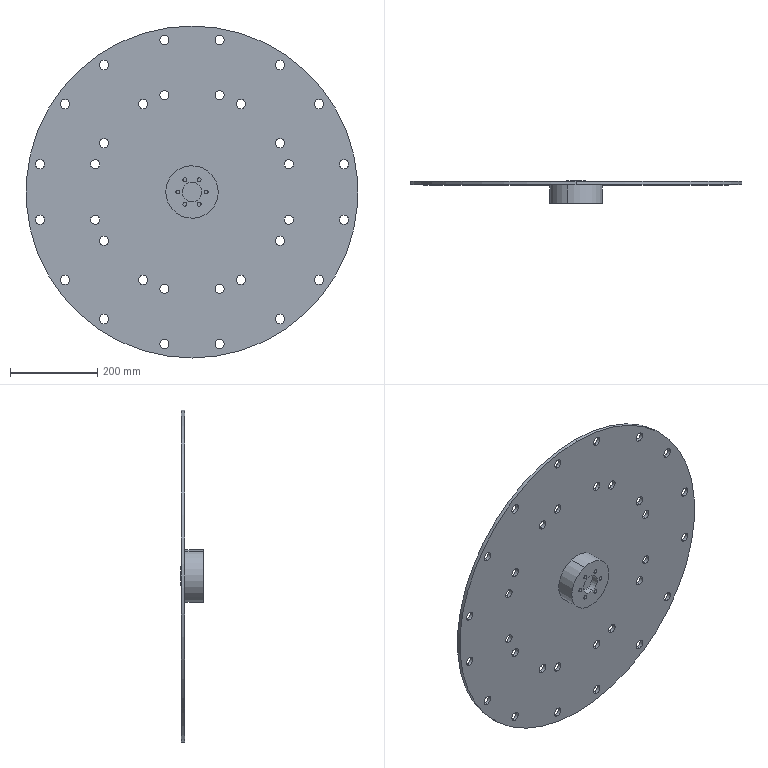Part | 2 solids | 317 faces | box 760 x 52.5 x 760 mm | volume 3968793 mm3 | cylinder 122 | spline 115 | plane 68 | cone 12 | commonest cylinder face diameters 21 x64 6.8 x12 8 x12 9 x12 15 x12 45 x4